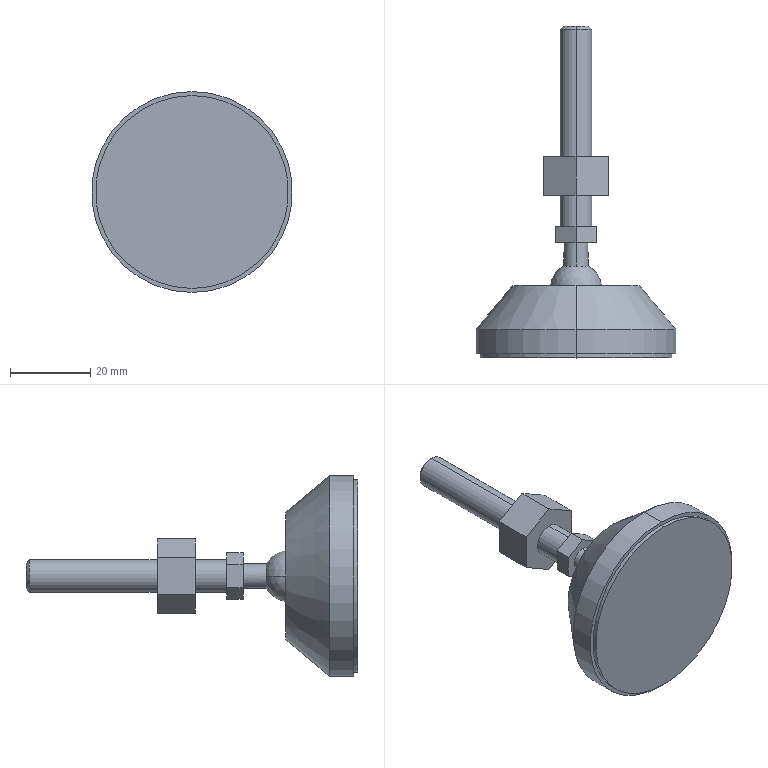Part | SolidWorks | features BaseBody 1 | 1 solid | 36 faces | box 50 x 82.6 x 50 mm | volume 33276 mm3 | plane 20 | cylinder 10 | cone 4 | sphere 2 | commonest cylinder face diameters 8 x4 6 x2 48 x2 50 x2
STEP:
#1=CARTESIAN_POINT('',(0.,7.,-25.));
#2=VERTEX_POINT('',#1);
#3=CARTESIAN_POINT('',(0.,7.,25.));
#4=VERTEX_POINT('',#3);
#5=CARTESIAN_POINT('',(0.,7.,0.));
#6=DIRECTION('',(0.,1.,0.));
#7=DIRECTION('',(0.,0.,1.));
#8=AXIS2_PLACEMENT_3D('',#5,#6,#7);
#9=CIRCLE('',#8,25.);
#10=EDGE_CURVE('',#2,#4,#9,.T.);
#11=ORIENTED_EDGE('',*,*,#10,.F.);
#12=CARTESIAN_POINT('',(0.,1.,-25.));
#13=VERTEX_POINT('',#12);
#14=CARTESIAN_POINT('',(0.,82.6,-25.));
#15=DIRECTION('',(0.,-1.,0.));
#16=VECTOR('',#15,1000.);
#17=LINE('',#14,#16);
#18=EDGE_CURVE('',#2,#13,#17,.T.);
#19=ORIENTED_EDGE('',*,*,#18,.T.);
#20=CARTESIAN_POINT('',(0.,1.,25.));
#21=VERTEX_POINT('',#20);
#22=CARTESIAN_POINT('',(0.,1.,0.));
#23=DIRECTION('',(0.,1.,0.));
#24=DIRECTION('',(0.,0.,1.));
#25=AXIS2_PLACEMENT_3D('',#22,#23,#24);
#26=CIRCLE('',#25,25.);
#27=EDGE_CURVE('',#13,#21,#26,.T.);
#28=ORIENTED_EDGE('',*,*,#27,.T.);
#29=CARTESIAN_POINT('',(0.,82.6,25.));
#30=DIRECTION('',(0.,-1.,0.));
#31=VECTOR('',#30,1000.);
#32=LINE('',#29,#31);
#33=EDGE_CURVE('',#4,#21,#32,.T.);
#34=ORIENTED_EDGE('',*,*,#33,.F.);
#35=EDGE_LOOP('',(#11,#19,#28,#34));
#36=FACE_OUTER_BOUND('',#35,.T.);
#37=CARTESIAN_POINT('',(0.,82.6,0.));
#38=DIRECTION('',(0.,-1.,0.));
#39=DIRECTION('',(0.,0.,1.));
#40=AXIS2_PLACEMENT_3D('',#37,#38,#39);
#41=CYLINDRICAL_SURFACE('',#40,25.);
#42=ADVANCED_FACE('',(#36),#41,.T.);
#43=CARTESIAN_POINT('',(0.,18.,15.77));
#44=VERTEX_POINT('',#43);
#45=CARTESIAN_POINT('',(0.,18.,-15.77));
#46=VERTEX_POINT('',#45);
#47=CARTESIAN_POINT('',(0.,18.,0.));
#48=DIRECTION('',(0.,1.,0.));
#49=DIRECTION('',(0.,0.,1.));
#50=AXIS2_PLACEMENT_3D('',#47,#48,#49);
#51=CIRCLE('',#50,15.77);
#52=EDGE_CURVE('',#44,#46,#51,.T.);
#53=ORIENTED_EDGE('',*,*,#52,.F.);
#54=CARTESIAN_POINT('',(0.,7.,25.));
#55=DIRECTION('',(0.,-0.766,0.6428));
#56=VECTOR('',#55,1000.);
#57=LINE('',#54,#56);
#58=EDGE_CURVE('',#44,#4,#57,.T.);
#59=ORIENTED_EDGE('',*,*,#58,.T.);
#60=CARTESIAN_POINT('',(0.,7.,0.));
#61=DIRECTION('',(0.,1.,0.));
#62=DIRECTION('',(0.,0.,1.));
#63=AXIS2_PLACEMENT_3D('',#60,#61,#62);
#64=CIRCLE('',#63,25.);
#65=EDGE_CURVE('',#4,#2,#64,.T.);
#66=ORIENTED_EDGE('',*,*,#65,.T.);
#67=CARTESIAN_POINT('',(0.,7.,-25.));
#68=DIRECTION('',(0.,-0.766,-0.6428));
#69=VECTOR('',#68,1000.);
#70=LINE('',#67,#69);
#71=EDGE_CURVE('',#46,#2,#70,.T.);
#72=ORIENTED_EDGE('',*,*,#71,.F.);
#73=EDGE_LOOP('',(#53,#59,#66,#72));
#74=FACE_OUTER_BOUND('',#73,.T.);
#75=CARTESIAN_POINT('',(0.,7.,0.));
#76=DIRECTION('',(0.,-1.,0.));
#77=DIRECTION('',(0.,0.,-1.));
#78=AXIS2_PLACEMENT_3D('',#75,#76,#77);
#79=CONICAL_SURFACE('',#78,25.,0.6981);
#80=ADVANCED_FACE('',(#74),#79,.T.);
#81=CARTESIAN_POINT('',(-6.35,18.,0.));
#82=VERTEX_POINT('',#81);
#83=CARTESIAN_POINT('',(6.35,18.,0.));
#84=VERTEX_POINT('',#83);
#85=CARTESIAN_POINT('',(0.,18.,0.));
#86=DIRECTION('',(0.,1.,0.));
#87=DIRECTION('',(0.,0.,1.));
#88=AXIS2_PLACEMENT_3D('',#85,#86,#87);
#89=CIRCLE('',#88,6.35);
#90=EDGE_CURVE('',#82,#84,#89,.T.);
#91=ORIENTED_EDGE('',*,*,#90,.T.);
#92=CARTESIAN_POINT('',(3.,22.853,0.));
#93=VERTEX_POINT('',#92);
#94=CARTESIAN_POINT('',(0.,17.2,0.));
#95=DIRECTION('',(0.,0.,1.));
#96=DIRECTION('',(1.,0.,0.));
#97=AXIS2_PLACEMENT_3D('',#94,#95,#96);
#98=CIRCLE('',#97,6.4);
#99=EDGE_CURVE('',#84,#93,#98,.T.);
#100=ORIENTED_EDGE('',*,*,#99,.T.);
#101=CARTESIAN_POINT('',(0.,22.853,3.));
#102=VERTEX_POINT('',#101);
#103=CARTESIAN_POINT('',(0.,22.853,0.));
#104=DIRECTION('',(0.,1.,0.));
#105=DIRECTION('',(0.,0.,1.));
#106=AXIS2_PLACEMENT_3D('',#103,#104,#105);
#107=CIRCLE('',#106,3.);
#108=EDGE_CURVE('',#102,#93,#107,.T.);
#109=ORIENTED_EDGE('',*,*,#108,.F.);
#110=CARTESIAN_POINT('',(-3.,22.853,0.));
#111=VERTEX_POINT('',#110);
#112=CARTESIAN_POINT('',(0.,22.853,0.));
#113=DIRECTION('',(0.,1.,0.));
#114=DIRECTION('',(0.,0.,1.));
#115=AXIS2_PLACEMENT_3D('',#112,#113,#114);
#116=CIRCLE('',#115,3.);
#117=EDGE_CURVE('',#111,#102,#116,.T.);
#118=ORIENTED_EDGE('',*,*,#117,.F.);
#119=CARTESIAN_POINT('',(0.,17.2,0.));
#120=DIRECTION('',(0.,0.,-1.));
#121=DIRECTION('',(-1.,0.,0.));
#122=AXIS2_PLACEMENT_3D('',#119,#120,#121);
#123=CIRCLE('',#122,6.4);
#124=EDGE_CURVE('',#82,#111,#123,.T.);
#125=ORIENTED_EDGE('',*,*,#124,.F.);
#126=EDGE_LOOP('',(#91,#100,#109,#118,#125));
#127=FACE_OUTER_BOUND('',#126,.T.);
#128=CARTESIAN_POINT('',(0.,17.2,0.));
#129=DIRECTION('',(0.,0.,1.));
#130=DIRECTION('',(-1.,0.,0.));
#131=AXIS2_PLACEMENT_3D('',#128,#129,#130);
#132=SPHERICAL_SURFACE('',#131,6.4);
#133=ADVANCED_FACE('',(#127),#132,.T.);
#134=CARTESIAN_POINT('',(0.,28.6,-3.));
#135=VERTEX_POINT('',#134);
#136=CARTESIAN_POINT('',(0.,28.6,3.));
#137=VERTEX_POINT('',#136);
#138=CARTESIAN_POINT('',(0.,28.6,0.));
#139=DIRECTION('',(0.,1.,0.));
#140=DIRECTION('',(0.,0.,1.));
#141=AXIS2_PLACEMENT_3D('',#138,#139,#140);
#142=CIRCLE('',#141,3.);
#143=EDGE_CURVE('',#135,#137,#142,.T.);
#144=ORIENTED_EDGE('',*,*,#143,.F.);
#145=CARTESIAN_POINT('',(0.,22.853,-3.));
#146=VERTEX_POINT('',#145);
#147=CARTESIAN_POINT('',(0.,82.6,-3.));
#148=DIRECTION('',(0.,-1.,0.));
#149=VECTOR('',#148,1000.);
#150=LINE('',#147,#149);
#151=EDGE_CURVE('',#135,#146,#150,.T.);
#152=ORIENTED_EDGE('',*,*,#151,.T.);
#153=CARTESIAN_POINT('',(0.,22.853,0.));
#154=DIRECTION('',(0.,1.,0.));
#155=DIRECTION('',(0.,0.,1.));
#156=AXIS2_PLACEMENT_3D('',#153,#154,#155);
#157=CIRCLE('',#156,3.);
#158=EDGE_CURVE('',#146,#111,#157,.T.);
#159=ORIENTED_EDGE('',*,*,#158,.T.);
#160=ORIENTED_EDGE('',*,*,#117,.T.);
#161=CARTESIAN_POINT('',(0.,82.6,3.));
#162=DIRECTION('',(0.,-1.,0.));
#163=VECTOR('',#162,1000.);
#164=LINE('',#161,#163);
#165=EDGE_CURVE('',#137,#102,#164,.T.);
#166=ORIENTED_EDGE('',*,*,#165,.F.);
#167=EDGE_LOOP('',(#144,#152,#159,#160,#166));
#168=FACE_OUTER_BOUND('',#167,.T.);
#169=CARTESIAN_POINT('',(0.,82.6,0.));
#170=DIRECTION('',(0.,-1.,0.));
#171=DIRECTION('',(0.,0.,1.));
#172=AXIS2_PLACEMENT_3D('',#169,#170,#171);
#173=CYLINDRICAL_SURFACE('',#172,3.);
#174=ADVANCED_FACE('',(#168),#173,.T.);
#175=CARTESIAN_POINT('',(0.,82.6,3.233));
#176=VERTEX_POINT('',#175);
#177=CARTESIAN_POINT('',(0.,82.6,-3.233));
#178=VERTEX_POINT('',#177);
#179=CARTESIAN_POINT('',(0.,82.6,0.));
#180=DIRECTION('',(0.,1.,0.));
#181=DIRECTION('',(0.,0.,1.));
#182=AXIS2_PLACEMENT_3D('',#179,#180,#181);
#183=CIRCLE('',#182,3.233);
#184=EDGE_CURVE('',#176,#178,#183,.T.);
#185=ORIENTED_EDGE('',*,*,#184,.F.);
#186=CARTESIAN_POINT('',(0.,81.833,4.));
#187=VERTEX_POINT('',#186);
#188=CARTESIAN_POINT('',(0.,81.833,4.));
#189=DIRECTION('',(0.,-0.7071,0.7071));
#190=VECTOR('',#189,1000.);
#191=LINE('',#188,#190);
#192=EDGE_CURVE('',#176,#187,#191,.T.);
#193=ORIENTED_EDGE('',*,*,#192,.T.);
#194=CARTESIAN_POINT('',(0.,81.833,-4.));
#195=VERTEX_POINT('',#194);
#196=CARTESIAN_POINT('',(0.,81.833,0.));
#197=DIRECTION('',(0.,1.,0.));
#198=DIRECTION('',(0.,0.,1.));
#199=AXIS2_PLACEMENT_3D('',#196,#197,#198);
#200=CIRCLE('',#199,4.);
#201=EDGE_CURVE('',#187,#195,#200,.T.);
#202=ORIENTED_EDGE('',*,*,#201,.T.);
#203=CARTESIAN_POINT('',(0.,81.833,-4.));
#204=DIRECTION('',(0.,-0.7071,-0.7071));
#205=VECTOR('',#204,1000.);
#206=LINE('',#203,#205);
#207=EDGE_CURVE('',#178,#195,#206,.T.);
#208=ORIENTED_EDGE('',*,*,#207,.F.);
#209=EDGE_LOOP('',(#185,#193,#202,#208));
#210=FACE_OUTER_BOUND('',#209,.T.);
#211=CARTESIAN_POINT('',(0.,81.833,0.));
#212=DIRECTION('',(0.,-1.,0.));
#213=DIRECTION('',(0.,0.,-1.));
#214=AXIS2_PLACEMENT_3D('',#211,#212,#213);
#215=CONICAL_SURFACE('',#214,4.,0.7854);
#216=ADVANCED_FACE('',(#210),#215,.T.);
#217=CARTESIAN_POINT('',(0.,81.833,0.));
#218=DIRECTION('',(0.,1.,0.));
#219=DIRECTION('',(0.,0.,1.));
#220=AXIS2_PLACEMENT_3D('',#217,#218,#219);
#221=CIRCLE('',#220,4.);
#222=EDGE_CURVE('',#195,#187,#221,.T.);
#223=ORIENTED_EDGE('',*,*,#222,.F.);
#224=CARTESIAN_POINT('',(0.,50.,-4.));
#225=VERTEX_POINT('',#224);
#226=CARTESIAN_POINT('',(0.,82.6,-4.));
#227=DIRECTION('',(0.,-1.,0.));
#228=VECTOR('',#227,1000.);
#229=LINE('',#226,#228);
#230=EDGE_CURVE('',#195,#225,#229,.T.);
#231=ORIENTED_EDGE('',*,*,#230,.T.);
#232=CARTESIAN_POINT('',(0.,50.,4.));
#233=VERTEX_POINT('',#232);
#234=CARTESIAN_POINT('',(0.,50.,0.));
#235=DIRECTION('',(0.,1.,0.));
#236=DIRECTION('',(1.,0.,0.));
#237=AXIS2_PLACEMENT_3D('',#234,#235,#236);
#238=CIRCLE('',#237,4.);
#239=EDGE_CURVE('',#225,#233,#238,.T.);
#240=ORIENTED_EDGE('',*,*,#239,.T.);
#241=CARTESIAN_POINT('',(0.,82.6,4.));
#242=DIRECTION('',(0.,-1.,0.));
#243=VECTOR('',#242,1000.);
#244=LINE('',#241,#243);
#245=EDGE_CURVE('',#187,#233,#244,.T.);
#246=ORIENTED_EDGE('',*,*,#245,.F.);
#247=EDGE_LOOP('',(#223,#231,#240,#246));
#248=FACE_OUTER_BOUND('',#247,.T.);
#249=CARTESIAN_POINT('',(0.,82.6,0.));
#250=DIRECTION('',(0.,-1.,0.));
#251=DIRECTION('',(0.,0.,1.));
#252=AXIS2_PLACEMENT_3D('',#249,#250,#251);
#253=CYLINDRICAL_SURFACE('',#252,4.);
#254=ADVANCED_FACE('',(#248),#253,.T.);
#255=CARTESIAN_POINT('',(0.,40.5,-4.));
#256=VERTEX_POINT('',#255);
#257=CARTESIAN_POINT('',(0.,40.5,4.));
#258=VERTEX_POINT('',#257);
#259=CARTESIAN_POINT('',(0.,40.5,0.));
#260=DIRECTION('',(0.,1.,0.));
#261=DIRECTION('',(1.,0.,0.));
#262=AXIS2_PLACEMENT_3D('',#259,#260,#261);
#263=CIRCLE('',#262,4.);
#264=EDGE_CURVE('',#256,#258,#263,.T.);
#265=ORIENTED_EDGE('',*,*,#264,.F.);
#266=CARTESIAN_POINT('',(0.,32.6,-4.));
#267=VERTEX_POINT('',#266);
#268=CARTESIAN_POINT('',(0.,82.6,-4.));
#269=DIRECTION('',(0.,-1.,0.));
#270=VECTOR('',#269,1000.);
#271=LINE('',#268,#270);
#272=EDGE_CURVE('',#256,#267,#271,.T.);
#273=ORIENTED_EDGE('',*,*,#272,.T.);
#274=CARTESIAN_POINT('',(0.,32.6,4.));
#275=VERTEX_POINT('',#274);
#276=CARTESIAN_POINT('',(0.,32.6,0.));
#277=DIRECTION('',(0.,1.,0.));
#278=DIRECTION('',(0.,0.,1.));
#279=AXIS2_PLACEMENT_3D('',#276,#277,#278);
#280=CIRCLE('',#279,4.);
#281=EDGE_CURVE('',#267,#275,#280,.T.);
#282=ORIENTED_EDGE('',*,*,#281,.T.);
#283=CARTESIAN_POINT('',(0.,82.6,4.));
#284=DIRECTION('',(0.,-1.,0.));
#285=VECTOR('',#284,1000.);
#286=LINE('',#283,#285);
#287=EDGE_CURVE('',#258,#275,#286,.T.);
#288=ORIENTED_EDGE('',*,*,#287,.F.);
#289=EDGE_LOOP('',(#265,#273,#282,#288));
#290=FACE_OUTER_BOUND('',#289,.T.);
#291=CARTESIAN_POINT('',(0.,82.6,0.));
#292=DIRECTION('',(0.,-1.,0.));
#293=DIRECTION('',(0.,0.,1.));
#294=AXIS2_PLACEMENT_3D('',#291,#292,#293);
#295=CYLINDRICAL_SURFACE('',#294,4.);
#296=ADVANCED_FACE('',(#290),#295,.T.);
#297=CARTESIAN_POINT('',(0.,1.,-24.));
#298=VERTEX_POINT('',#297);
#299=CARTESIAN_POINT('',(0.,1.,24.));
#300=VERTEX_POINT('',#299);
#301=CARTESIAN_POINT('',(0.,1.,0.));
#302=DIRECTION('',(0.,1.,0.));
#303=DIRECTION('',(0.,0.,1.));
#304=AXIS2_PLACEMENT_3D('',#301,#302,#303);
#305=CIRCLE('',#304,24.);
#306=EDGE_CURVE('',#298,#300,#305,.T.);
#307=ORIENTED_EDGE('',*,*,#306,.F.);
#308=CARTESIAN_POINT('',(0.,0.,-24.));
#309=VERTEX_POINT('',#308);
#310=CARTESIAN_POINT('',(0.,82.6,-24.));
#311=DIRECTION('',(0.,-1.,0.));
#312=VECTOR('',#311,1000.);
#313=LINE('',#310,#312);
#314=EDGE_CURVE('',#298,#309,#313,.T.);
#315=ORIENTED_EDGE('',*,*,#314,.T.);
#316=CARTESIAN_POINT('',(0.,0.,24.));
#317=VERTEX_POINT('',#316);
#318=CARTESIAN_POINT('',(0.,0.,0.));
#319=DIRECTION('',(0.,1.,0.));
#320=DIRECTION('',(0.,0.,1.));
#321=AXIS2_PLACEMENT_3D('',#318,#319,#320);
#322=CIRCLE('',#321,24.);
#323=EDGE_CURVE('',#309,#317,#322,.T.);
#324=ORIENTED_EDGE('',*,*,#323,.T.);
#325=CARTESIAN_POINT('',(0.,82.6,24.));
#326=DIRECTION('',(0.,-1.,0.));
#327=VECTOR('',#326,1000.);
#328=LINE('',#325,#327);
#329=EDGE_CURVE('',#300,#317,#328,.T.);
#330=ORIENTED_EDGE('',*,*,#329,.F.);
#331=EDGE_LOOP('',(#307,#315,#324,#330));
#332=FACE_OUTER_BOUND('',#331,.T.);
#333=CARTESIAN_POINT('',(0.,82.6,0.));
#334=DIRECTION('',(0.,-1.,0.));
#335=DIRECTION('',(0.,0.,1.));
#336=AXIS2_PLACEMENT_3D('',#333,#334,#335);
#337=CYLINDRICAL_SURFACE('',#336,24.);
#338=ADVANCED_FACE('',(#332),#337,.T.);
#339=CARTESIAN_POINT('',(0.,0.,0.));
#340=DIRECTION('',(0.,1.,0.));
#341=DIRECTION('',(0.,0.,1.));
#342=AXIS2_PLACEMENT_3D('',#339,#340,#341);
#343=CIRCLE('',#342,24.);
#344=EDGE_CURVE('',#317,#309,#343,.T.);
#345=ORIENTED_EDGE('',*,*,#344,.F.);
#346=ORIENTED_EDGE('',*,*,#323,.F.);
#347=EDGE_LOOP('',(#345,#346));
#348=FACE_OUTER_BOUND('',#347,.T.);
#349=CARTESIAN_POINT('',(0.,0.,0.));
#350=DIRECTION('',(0.,1.,0.));
#351=DIRECTION('',(1.,0.,0.));
#352=AXIS2_PLACEMENT_3D('',#349,#350,#351);
#353=PLANE('',#352);
#354=ADVANCED_FACE('',(#348),#353,.F.);
#355=ORIENTED_EDGE('',*,*,#314,.F.);
#356=CARTESIAN_POINT('',(0.,1.,0.));
#357=DIRECTION('',(0.,1.,0.));
#358=DIRECTION('',(0.,0.,1.));
#359=AXIS2_PLACEMENT_3D('',#356,#357,#358);
#360=CIRCLE('',#359,24.);
#361=EDGE_CURVE('',#300,#298,#360,.T.);
#362=ORIENTED_EDGE('',*,*,#361,.F.);
#363=ORIENTED_EDGE('',*,*,#329,.T.);
#364=ORIENTED_EDGE('',*,*,#344,.T.);
#365=EDGE_LOOP('',(#355,#362,#363,#364));
#366=FACE_OUTER_BOUND('',#365,.T.);
#367=CARTESIAN_POINT('',(0.,82.6,0.));
#368=DIRECTION('',(0.,-1.,0.));
#369=DIRECTION('',(0.,0.,1.));
#370=AXIS2_PLACEMENT_3D('',#367,#368,#369);
#371=CYLINDRICAL_SURFACE('',#370,24.);
#372=ADVANCED_FACE('',(#366),#371,.T.);
#373=CARTESIAN_POINT('',(-5.,28.6,2.887));
#374=VERTEX_POINT('',#373);
#375=CARTESIAN_POINT('',(0.,28.6,5.774));
#376=VERTEX_POINT('',#375);
#377=CARTESIAN_POINT('',(-5.,28.6,2.887));
#378=DIRECTION('',(0.866,0.,0.5));
#379=VECTOR('',#378,1000.);
#380=LINE('',#377,#379);
#381=EDGE_CURVE('',#374,#376,#380,.T.);
#382=ORIENTED_EDGE('',*,*,#381,.F.);
#383=CARTESIAN_POINT('',(-5.,28.6,-2.887));
#384=VERTEX_POINT('',#383);
#385=CARTESIAN_POINT('',(-5.,28.6,-2.887));
#386=DIRECTION('',(0.,0.,1.));
#387=VECTOR('',#386,1000.);
#388=LINE('',#385,#387);
#389=EDGE_CURVE('',#384,#374,#388,.T.);
#390=ORIENTED_EDGE('',*,*,#389,.F.);
#391=CARTESIAN_POINT('',(0.,28.6,-5.774));
#392=VERTEX_POINT('',#391);
#393=CARTESIAN_POINT('',(0.,28.6,-5.774));
#394=DIRECTION('',(-0.866,0.,0.5));
#395=VECTOR('',#394,1000.);
#396=LINE('',#393,#395);
#397=EDGE_CURVE('',#392,#384,#396,.T.);
#398=ORIENTED_EDGE('',*,*,#397,.F.);
#399=CARTESIAN_POINT('',(5.,28.6,-2.887));
#400=VERTEX_POINT('',#399);
#401=CARTESIAN_POINT('',(5.,28.6,-2.887));
#402=DIRECTION('',(-0.866,0.,-0.5));
#403=VECTOR('',#402,1000.);
#404=LINE('',#401,#403);
#405=EDGE_CURVE('',#400,#392,#404,.T.);
#406=ORIENTED_EDGE('',*,*,#405,.F.);
#407=CARTESIAN_POINT('',(5.,28.6,2.887));
#408=VERTEX_POINT('',#407);
#409=CARTESIAN_POINT('',(5.,28.6,2.887));
#410=DIRECTION('',(0.,0.,-1.));
#411=VECTOR('',#410,1000.);
#412=LINE('',#409,#411);
#413=EDGE_CURVE('',#408,#400,#412,.T.);
#414=ORIENTED_EDGE('',*,*,#413,.F.);
#415=CARTESIAN_POINT('',(0.,28.6,5.774));
#416=DIRECTION('',(0.866,0.,-0.5));
#417=VECTOR('',#416,1000.);
#418=LINE('',#415,#417);
#419=EDGE_CURVE('',#376,#408,#418,.T.);
#420=ORIENTED_EDGE('',*,*,#419,.F.);
#421=EDGE_LOOP('',(#382,#390,#398,#406,#414,#420));
#422=FACE_OUTER_BOUND('',#421,.T.);
#423=CARTESIAN_POINT('',(0.,28.6,0.));
#424=DIRECTION('',(0.,1.,0.));
#425=DIRECTION('',(0.,0.,1.));
#426=AXIS2_PLACEMENT_3D('',#423,#424,#425);
#427=CIRCLE('',#426,3.);
#428=EDGE_CURVE('',#137,#135,#427,.T.);
#429=ORIENTED_EDGE('',*,*,#428,.T.);
#430=ORIENTED_EDGE('',*,*,#143,.T.);
#431=EDGE_LOOP('',(#429,#430));
#432=FACE_BOUND('',#431,.T.);
#433=CARTESIAN_POINT('',(-3.,28.6,0.));
#434=DIRECTION('',(0.,1.,0.));
#435=DIRECTION('',(1.,0.,0.));
#436=AXIS2_PLACEMENT_3D('',#433,#434,#435);
#437=PLANE('',#436);
#438=ADVANCED_FACE('',(#422,#432),#437,.F.);
#439=ORIENTED_EDGE('',*,*,#272,.F.);
#440=CARTESIAN_POINT('',(0.,40.5,0.));
#441=DIRECTION('',(0.,1.,0.));
#442=DIRECTION('',(1.,0.,0.));
#443=AXIS2_PLACEMENT_3D('',#440,#441,#442);
#444=CIRCLE('',#443,4.);
#445=EDGE_CURVE('',#258,#256,#444,.T.);
#446=ORIENTED_EDGE('',*,*,#445,.F.);
#447=ORIENTED_EDGE('',*,*,#287,.T.);
#448=CARTESIAN_POINT('',(0.,32.6,0.));
#449=DIRECTION('',(0.,1.,0.));
#450=DIRECTION('',(0.,0.,1.));
#451=AXIS2_PLACEMENT_3D('',#448,#449,#450);
#452=CIRCLE('',#451,4.);
#453=EDGE_CURVE('',#275,#267,#452,.T.);
#454=ORIENTED_EDGE('',*,*,#453,.T.);
#455=EDGE_LOOP('',(#439,#446,#447,#454));
#456=FACE_OUTER_BOUND('',#455,.T.);
#457=CARTESIAN_POINT('',(0.,82.6,0.));
#458=DIRECTION('',(0.,-1.,0.));
#459=DIRECTION('',(0.,0.,1.));
#460=AXIS2_PLACEMENT_3D('',#457,#458,#459);
#461=CYLINDRICAL_SURFACE('',#460,4.);
#462=ADVANCED_FACE('',(#456),#461,.T.);
#463=ORIENTED_EDGE('',*,*,#230,.F.);
#464=ORIENTED_EDGE('',*,*,#201,.F.);
#465=ORIENTED_EDGE('',*,*,#245,.T.);
#466=CARTESIAN_POINT('',(0.,50.,0.));
#467=DIRECTION('',(0.,1.,0.));
#468=DIRECTION('',(1.,0.,0.));
#469=AXIS2_PLACEMENT_3D('',#466,#467,#468);
#470=CIRCLE('',#469,4.);
#471=EDGE_CURVE('',#233,#225,#470,.T.);
#472=ORIENTED_EDGE('',*,*,#471,.T.);
#473=EDGE_LOOP('',(#463,#464,#465,#472));
#474=FACE_OUTER_BOUND('',#473,.T.);
#475=CARTESIAN_POINT('',(0.,82.6,0.));
#476=DIRECTION('',(0.,-1.,0.));
#477=DIRECTION('',(0.,0.,1.));
#478=AXIS2_PLACEMENT_3D('',#475,#476,#477);
#479=CYLINDRICAL_SURFACE('',#478,4.);
#480=ADVANCED_FACE('',(#474),#479,.T.);
#481=ORIENTED_EDGE('',*,*,#192,.F.);
#482=CARTESIAN_POINT('',(0.,82.6,0.));
#483=DIRECTION('',(0.,1.,0.));
#484=DIRECTION('',(0.,0.,1.));
#485=AXIS2_PLACEMENT_3D('',#482,#483,#484);
#486=CIRCLE('',#485,3.233);
#487=EDGE_CURVE('',#178,#176,#486,.T.);
#488=ORIENTED_EDGE('',*,*,#487,.F.);
#489=ORIENTED_EDGE('',*,*,#207,.T.);
#490=ORIENTED_EDGE('',*,*,#222,.T.);
#491=EDGE_LOOP('',(#481,#488,#489,#490));
#492=FACE_OUTER_BOUND('',#491,.T.);
#493=CARTESIAN_POINT('',(0.,81.833,0.));
#494=DIRECTION('',(0.,-1.,0.));
#495=DIRECTION('',(0.,0.,-1.));
#496=AXIS2_PLACEMENT_3D('',#493,#494,#495);
#497=CONICAL_SURFACE('',#496,4.,0.7854);
#498=ADVANCED_FACE('',(#492),#497,.T.);
#499=CARTESIAN_POINT('',(-8.,50.,-4.619));
#500=VERTEX_POINT('',#499);
#501=CARTESIAN_POINT('',(-8.,50.,4.619));
#502=VERTEX_POINT('',#501);
#503=CARTESIAN_POINT('',(-8.,50.,-4.619));
#504=DIRECTION('',(0.,0.,1.));
#505=VECTOR('',#504,1000.);
#506=LINE('',#503,#505);
#507=EDGE_CURVE('',#500,#502,#506,.T.);
#508=ORIENTED_EDGE('',*,*,#507,.T.);
#509=CARTESIAN_POINT('',(0.,50.,9.238));
#510=VERTEX_POINT('',#509);
#511=CARTESIAN_POINT('',(-8.,50.,4.619));
#512=DIRECTION('',(0.866,0.,0.5));
#513=VECTOR('',#512,1000.);
#514=LINE('',#511,#513);
#515=EDGE_CURVE('',#502,#510,#514,.T.);
#516=ORIENTED_EDGE('',*,*,#515,.T.);
#517=CARTESIAN_POINT('',(8.,50.,4.619));
#518=VERTEX_POINT('',#517);
#519=CARTESIAN_POINT('',(0.,50.,9.238));
#520=DIRECTION('',(0.866,0.,-0.5));
#521=VECTOR('',#520,1000.);
#522=LINE('',#519,#521);
#523=EDGE_CURVE('',#510,#518,#522,.T.);
#524=ORIENTED_EDGE('',*,*,#523,.T.);
#525=CARTESIAN_POINT('',(8.,50.,-4.619));
#526=VERTEX_POINT('',#525);
#527=CARTESIAN_POINT('',(8.,50.,4.619));
#528=DIRECTION('',(0.,0.,-1.));
#529=VECTOR('',#528,1000.);
#530=LINE('',#527,#529);
#531=EDGE_CURVE('',#518,#526,#530,.T.);
#532=ORIENTED_EDGE('',*,*,#531,.T.);
#533=CARTESIAN_POINT('',(0.,50.,-9.238));
#534=VERTEX_POINT('',#533);
#535=CARTESIAN_POINT('',(8.,50.,-4.619));
#536=DIRECTION('',(-0.866,0.,-0.5));
#537=VECTOR('',#536,1000.);
#538=LINE('',#535,#537);
#539=EDGE_CURVE('',#526,#534,#538,.T.);
#540=ORIENTED_EDGE('',*,*,#539,.T.);
#541=CARTESIAN_POINT('',(0.,50.,-9.238));
#542=DIRECTION('',(-0.866,0.,0.5));
#543=VECTOR('',#542,1000.);
#544=LINE('',#541,#543);
#545=EDGE_CURVE('',#534,#500,#544,.T.);
#546=ORIENTED_EDGE('',*,*,#545,.T.);
#547=EDGE_LOOP('',(#508,#516,#524,#532,#540,#546));
#548=FACE_OUTER_BOUND('',#547,.T.);
#549=ORIENTED_EDGE('',*,*,#471,.F.);
#550=ORIENTED_EDGE('',*,*,#239,.F.);
#551=EDGE_LOOP('',(#549,#550));
#552=FACE_BOUND('',#551,.T.);
#553=CARTESIAN_POINT('',(0.,50.,0.));
#554=DIRECTION('',(0.,1.,0.));
#555=DIRECTION('',(1.,0.,0.));
#556=AXIS2_PLACEMENT_3D('',#553,#554,#555);
#557=PLANE('',#556);
#558=ADVANCED_FACE('',(#548,#552),#557,.T.);
#559=ORIENTED_EDGE('',*,*,#523,.F.);
#560=CARTESIAN_POINT('',(0.,40.5,9.238));
#561=VERTEX_POINT('',#560);
#562=CARTESIAN_POINT('',(0.,40.5,9.238));
#563=DIRECTION('',(0.,1.,0.));
#564=VECTOR('',#563,1000.);
#565=LINE('',#562,#564);
#566=EDGE_CURVE('',#561,#510,#565,.T.);
#567=ORIENTED_EDGE('',*,*,#566,.F.);
#568=CARTESIAN_POINT('',(8.,40.5,4.619));
#569=VERTEX_POINT('',#568);
#570=CARTESIAN_POINT('',(0.,40.5,9.238));
#571=DIRECTION('',(0.866,0.,-0.5));
#572=VECTOR('',#571,1000.);
#573=LINE('',#570,#572);
#574=EDGE_CURVE('',#561,#569,#573,.T.);
#575=ORIENTED_EDGE('',*,*,#574,.T.);
#576=CARTESIAN_POINT('',(8.,40.5,4.619));
#577=DIRECTION('',(0.,1.,0.));
#578=VECTOR('',#577,1000.);
#579=LINE('',#576,#578);
#580=EDGE_CURVE('',#569,#518,#579,.T.);
#581=ORIENTED_EDGE('',*,*,#580,.T.);
#582=EDGE_LOOP('',(#559,#567,#575,#581));
#583=FACE_OUTER_BOUND('',#582,.T.);
#584=CARTESIAN_POINT('',(0.,40.5,9.238));
#585=DIRECTION('',(0.5,0.,0.866));
#586=DIRECTION('',(0.,-1.,0.));
#587=AXIS2_PLACEMENT_3D('',#584,#585,#586);
#588=PLANE('',#587);
#589=ADVANCED_FACE('',(#583),#588,.T.);
#590=ORIENTED_EDGE('',*,*,#531,.F.);
#591=ORIENTED_EDGE('',*,*,#580,.F.);
#592=CARTESIAN_POINT('',(8.,40.5,-4.619));
#593=VERTEX_POINT('',#592);
#594=CARTESIAN_POINT('',(8.,40.5,4.619));
#595=DIRECTION('',(0.,0.,-1.));
#596=VECTOR('',#595,1000.);
#597=LINE('',#594,#596);
#598=EDGE_CURVE('',#569,#593,#597,.T.);
#599=ORIENTED_EDGE('',*,*,#598,.T.);
#600=CARTESIAN_POINT('',(8.,40.5,-4.619));
#601=DIRECTION('',(0.,1.,0.));
#602=VECTOR('',#601,1000.);
#603=LINE('',#600,#602);
#604=EDGE_CURVE('',#593,#526,#603,.T.);
#605=ORIENTED_EDGE('',*,*,#604,.T.);
#606=EDGE_LOOP('',(#590,#591,#599,#605));
#607=FACE_OUTER_BOUND('',#606,.T.);
#608=CARTESIAN_POINT('',(8.,40.5,4.619));
#609=DIRECTION('',(1.,0.,0.));
#610=DIRECTION('',(0.,1.,0.));
#611=AXIS2_PLACEMENT_3D('',#608,#609,#610);
#612=PLANE('',#611);
#613=ADVANCED_FACE('',(#607),#612,.T.);
#614=ORIENTED_EDGE('',*,*,#515,.F.);
#615=CARTESIAN_POINT('',(-8.,40.5,4.619));
#616=VERTEX_POINT('',#615);
#617=CARTESIAN_POINT('',(-8.,40.5,4.619));
#618=DIRECTION('',(0.,1.,0.));
#619=VECTOR('',#618,1000.);
#620=LINE('',#617,#619);
#621=EDGE_CURVE('',#616,#502,#620,.T.);
#622=ORIENTED_EDGE('',*,*,#621,.F.);
#623=CARTESIAN_POINT('',(-8.,40.5,4.619));
#624=DIRECTION('',(0.866,0.,0.5));
#625=VECTOR('',#624,1000.);
#626=LINE('',#623,#625);
#627=EDGE_CURVE('',#616,#561,#626,.T.);
#628=ORIENTED_EDGE('',*,*,#627,.T.);
#629=ORIENTED_EDGE('',*,*,#566,.T.);
#630=EDGE_LOOP('',(#614,#622,#628,#629));
#631=FACE_OUTER_BOUND('',#630,.T.);
#632=CARTESIAN_POINT('',(-8.,40.5,4.619));
#633=DIRECTION('',(-0.5,0.,0.866));
#634=DIRECTION('',(0.,1.,0.));
#635=AXIS2_PLACEMENT_3D('',#632,#633,#634);
#636=PLANE('',#635);
#637=ADVANCED_FACE('',(#631),#636,.T.);
#638=ORIENTED_EDGE('',*,*,#507,.F.);
#639=CARTESIAN_POINT('',(-8.,40.5,-4.619));
#640=VERTEX_POINT('',#639);
#641=CARTESIAN_POINT('',(-8.,40.5,-4.619));
#642=DIRECTION('',(0.,1.,0.));
#643=VECTOR('',#642,1000.);
#644=LINE('',#641,#643);
#645=EDGE_CURVE('',#640,#500,#644,.T.);
#646=ORIENTED_EDGE('',*,*,#645,.F.);
#647=CARTESIAN_POINT('',(-8.,40.5,-4.619));
#648=DIRECTION('',(0.,0.,1.));
#649=VECTOR('',#648,1000.);
#650=LINE('',#647,#649);
#651=EDGE_CURVE('',#640,#616,#650,.T.);
#652=ORIENTED_EDGE('',*,*,#651,.T.);
#653=ORIENTED_EDGE('',*,*,#621,.T.);
#654=EDGE_LOOP('',(#638,#646,#652,#653));
#655=FACE_OUTER_BOUND('',#654,.T.);
#656=CARTESIAN_POINT('',(-8.,40.5,-4.619));
#657=DIRECTION('',(-1.,0.,0.));
#658=DIRECTION('',(0.,0.,1.));
#659=AXIS2_PLACEMENT_3D('',#656,#657,#658);
#660=PLANE('',#659);
#661=ADVANCED_FACE('',(#655),#660,.T.);
#662=CARTESIAN_POINT('',(5.,32.6,2.887));
#663=VERTEX_POINT('',#662);
#664=CARTESIAN_POINT('',(5.,32.6,-2.887));
#665=VERTEX_POINT('',#664);
#666=CARTESIAN_POINT('',(5.,32.6,2.887));
#667=DIRECTION('',(0.,0.,-1.));
#668=VECTOR('',#667,1000.);
#669=LINE('',#666,#668);
#670=EDGE_CURVE('',#663,#665,#669,.T.);
#671=ORIENTED_EDGE('',*,*,#670,.F.);
#672=CARTESIAN_POINT('',(5.,28.6,2.887));
#673=DIRECTION('',(0.,1.,0.));
#674=VECTOR('',#673,1000.);
#675=LINE('',#672,#674);
#676=EDGE_CURVE('',#408,#663,#675,.T.);
#677=ORIENTED_EDGE('',*,*,#676,.F.);
#678=ORIENTED_EDGE('',*,*,#413,.T.);
#679=CARTESIAN_POINT('',(5.,28.6,-2.887));
#680=DIRECTION('',(0.,1.,0.));
#681=VECTOR('',#680,1000.);
#682=LINE('',#679,#681);
#683=EDGE_CURVE('',#400,#665,#682,.T.);
#684=ORIENTED_EDGE('',*,*,#683,.T.);
#685=EDGE_LOOP('',(#671,#677,#678,#684));
#686=FACE_OUTER_BOUND('',#685,.T.);
#687=CARTESIAN_POINT('',(5.,28.6,2.887));
#688=DIRECTION('',(1.,0.,0.));
#689=DIRECTION('',(0.,1.,0.));
#690=AXIS2_PLACEMENT_3D('',#687,#688,#689);
#691=PLANE('',#690);
#692=ADVANCED_FACE('',(#686),#691,.T.);
#693=CARTESIAN_POINT('',(0.,32.6,5.774));
#694=VERTEX_POINT('',#693);
#695=CARTESIAN_POINT('',(0.,32.6,5.774));
#696=DIRECTION('',(0.866,0.,-0.5));
#697=VECTOR('',#696,1000.);
#698=LINE('',#695,#697);
#699=EDGE_CURVE('',#694,#663,#698,.T.);
#700=ORIENTED_EDGE('',*,*,#699,.F.);
#701=CARTESIAN_POINT('',(0.,28.6,5.774));
#702=DIRECTION('',(0.,1.,0.));
#703=VECTOR('',#702,1000.);
#704=LINE('',#701,#703);
#705=EDGE_CURVE('',#376,#694,#704,.T.);
#706=ORIENTED_EDGE('',*,*,#705,.F.);
#707=ORIENTED_EDGE('',*,*,#419,.T.);
#708=ORIENTED_EDGE('',*,*,#676,.T.);
#709=EDGE_LOOP('',(#700,#706,#707,#708));
#710=FACE_OUTER_BOUND('',#709,.T.);
#711=CARTESIAN_POINT('',(0.,28.6,5.774));
#712=DIRECTION('',(0.5,0.,0.866));
#713=DIRECTION('',(0.,-1.,0.));
#714=AXIS2_PLACEMENT_3D('',#711,#712,#713);
#715=PLANE('',#714);
#716=ADVANCED_FACE('',(#710),#715,.T.);
#717=CARTESIAN_POINT('',(-5.,32.6,2.887));
#718=VERTEX_POINT('',#717);
#719=CARTESIAN_POINT('',(-5.,32.6,2.887));
#720=DIRECTION('',(0.866,0.,0.5));
#721=VECTOR('',#720,1000.);
#722=LINE('',#719,#721);
#723=EDGE_CURVE('',#718,#694,#722,.T.);
#724=ORIENTED_EDGE('',*,*,#723,.F.);
#725=CARTESIAN_POINT('',(-5.,28.6,2.887));
#726=DIRECTION('',(0.,1.,0.));
#727=VECTOR('',#726,1000.);
#728=LINE('',#725,#727);
#729=EDGE_CURVE('',#374,#718,#728,.T.);
#730=ORIENTED_EDGE('',*,*,#729,.F.);
#731=ORIENTED_EDGE('',*,*,#381,.T.);
#732=ORIENTED_EDGE('',*,*,#705,.T.);
#733=EDGE_LOOP('',(#724,#730,#731,#732));
#734=FACE_OUTER_BOUND('',#733,.T.);
#735=CARTESIAN_POINT('',(-5.,28.6,2.887));
#736=DIRECTION('',(-0.5,0.,0.866));
#737=DIRECTION('',(0.,1.,0.));
#738=AXIS2_PLACEMENT_3D('',#735,#736,#737);
#739=PLANE('',#738);
#740=ADVANCED_FACE('',(#734),#739,.T.);
#741=CARTESIAN_POINT('',(-5.,32.6,-2.887));
#742=VERTEX_POINT('',#741);
#743=CARTESIAN_POINT('',(-5.,32.6,0.));
#744=DIRECTION('',(0.,0.,-1.));
#745=VECTOR('',#744,1000.);
#746=LINE('',#743,#745);
#747=EDGE_CURVE('',#718,#742,#746,.T.);
#748=ORIENTED_EDGE('',*,*,#747,.T.);
#749=CARTESIAN_POINT('',(-5.,28.6,-2.887));
#750=DIRECTION('',(0.,1.,0.));
#751=VECTOR('',#750,1000.);
#752=LINE('',#749,#751);
#753=EDGE_CURVE('',#384,#742,#752,.T.);
#754=ORIENTED_EDGE('',*,*,#753,.F.);
#755=ORIENTED_EDGE('',*,*,#389,.T.);
#756=ORIENTED_EDGE('',*,*,#729,.T.);
#757=EDGE_LOOP('',(#748,#754,#755,#756));
#758=FACE_OUTER_BOUND('',#757,.T.);
#759=CARTESIAN_POINT('',(-5.,28.6,-2.887));
#760=DIRECTION('',(-1.,0.,0.));
#761=DIRECTION('',(0.,0.,1.));
#762=AXIS2_PLACEMENT_3D('',#759,#760,#761);
#763=PLANE('',#762);
#764=ADVANCED_FACE('',(#758),#763,.T.);
#765=CARTESIAN_POINT('',(0.,32.6,-5.774));
#766=VERTEX_POINT('',#765);
#767=CARTESIAN_POINT('',(0.,32.6,-5.774));
#768=DIRECTION('',(-0.866,0.,0.5));
#769=VECTOR('',#768,1000.);
#770=LINE('',#767,#769);
#771=EDGE_CURVE('',#766,#742,#770,.T.);
#772=ORIENTED_EDGE('',*,*,#771,.F.);
#773=CARTESIAN_POINT('',(0.,28.6,-5.774));
#774=DIRECTION('',(0.,1.,0.));
#775=VECTOR('',#774,1000.);
#776=LINE('',#773,#775);
#777=EDGE_CURVE('',#392,#766,#776,.T.);
#778=ORIENTED_EDGE('',*,*,#777,.F.);
#779=ORIENTED_EDGE('',*,*,#397,.T.);
#780=ORIENTED_EDGE('',*,*,#753,.T.);
#781=EDGE_LOOP('',(#772,#778,#779,#780));
#782=FACE_OUTER_BOUND('',#781,.T.);
#783=CARTESIAN_POINT('',(0.,28.6,-5.774));
#784=DIRECTION('',(-0.5,0.,-0.866));
#785=DIRECTION('',(-0.866,0.,0.5));
#786=AXIS2_PLACEMENT_3D('',#783,#784,#785);
#787=PLANE('',#786);
#788=ADVANCED_FACE('',(#782),#787,.T.);
#789=CARTESIAN_POINT('',(5.,32.6,-2.887));
#790=DIRECTION('',(-0.866,0.,-0.5));
#791=VECTOR('',#790,1000.);
#792=LINE('',#789,#791);
#793=EDGE_CURVE('',#665,#766,#792,.T.);
#794=ORIENTED_EDGE('',*,*,#793,.F.);
#795=ORIENTED_EDGE('',*,*,#683,.F.);
#796=ORIENTED_EDGE('',*,*,#405,.T.);
#797=ORIENTED_EDGE('',*,*,#777,.T.);
#798=EDGE_LOOP('',(#794,#795,#796,#797));
#799=FACE_OUTER_BOUND('',#798,.T.);
#800=CARTESIAN_POINT('',(5.,28.6,-2.887));
#801=DIRECTION('',(0.5,0.,-0.866));
#802=DIRECTION('',(0.,-1.,0.));
#803=AXIS2_PLACEMENT_3D('',#800,#801,#802);
#804=PLANE('',#803);
#805=ADVANCED_FACE('',(#799),#804,.T.);
#806=ORIENTED_EDGE('',*,*,#487,.T.);
#807=ORIENTED_EDGE('',*,*,#184,.T.);
#808=EDGE_LOOP('',(#806,#807));
#809=FACE_OUTER_BOUND('',#808,.T.);
#810=CARTESIAN_POINT('',(-3.233,82.6,0.));
#811=DIRECTION('',(0.,-1.,0.));
#812=DIRECTION('',(0.,0.,-1.));
#813=AXIS2_PLACEMENT_3D('',#810,#811,#812);
#814=PLANE('',#813);
#815=ADVANCED_FACE('',(#809),#814,.F.);
#816=ORIENTED_EDGE('',*,*,#651,.F.);
#817=CARTESIAN_POINT('',(0.,40.5,-9.238));
#818=VERTEX_POINT('',#817);
#819=CARTESIAN_POINT('',(0.,40.5,-9.238));
#820=DIRECTION('',(-0.866,0.,0.5));
#821=VECTOR('',#820,1000.);
#822=LINE('',#819,#821);
#823=EDGE_CURVE('',#818,#640,#822,.T.);
#824=ORIENTED_EDGE('',*,*,#823,.F.);
#825=CARTESIAN_POINT('',(8.,40.5,-4.619));
#826=DIRECTION('',(-0.866,0.,-0.5));
#827=VECTOR('',#826,1000.);
#828=LINE('',#825,#827);
#829=EDGE_CURVE('',#593,#818,#828,.T.);
#830=ORIENTED_EDGE('',*,*,#829,.F.);
#831=ORIENTED_EDGE('',*,*,#598,.F.);
#832=ORIENTED_EDGE('',*,*,#574,.F.);
#833=ORIENTED_EDGE('',*,*,#627,.F.);
#834=EDGE_LOOP('',(#816,#824,#830,#831,#832,#833));
#835=FACE_OUTER_BOUND('',#834,.T.);
#836=ORIENTED_EDGE('',*,*,#445,.T.);
#837=ORIENTED_EDGE('',*,*,#264,.T.);
#838=EDGE_LOOP('',(#836,#837));
#839=FACE_BOUND('',#838,.T.);
#840=CARTESIAN_POINT('',(0.,40.5,0.));
#841=DIRECTION('',(0.,1.,0.));
#842=DIRECTION('',(1.,0.,0.));
#843=AXIS2_PLACEMENT_3D('',#840,#841,#842);
#844=PLANE('',#843);
#845=ADVANCED_FACE('',(#835,#839),#844,.F.);
#846=ORIENTED_EDGE('',*,*,#545,.F.);
#847=CARTESIAN_POINT('',(0.,40.5,-9.238));
#848=DIRECTION('',(0.,1.,0.));
#849=VECTOR('',#848,1000.);
#850=LINE('',#847,#849);
#851=EDGE_CURVE('',#818,#534,#850,.T.);
#852=ORIENTED_EDGE('',*,*,#851,.F.);
#853=ORIENTED_EDGE('',*,*,#823,.T.);
#854=ORIENTED_EDGE('',*,*,#645,.T.);
#855=EDGE_LOOP('',(#846,#852,#853,#854));
#856=FACE_OUTER_BOUND('',#855,.T.);
#857=CARTESIAN_POINT('',(0.,40.5,-9.238));
#858=DIRECTION('',(-0.5,0.,-0.866));
#859=DIRECTION('',(-0.866,0.,0.5));
#860=AXIS2_PLACEMENT_3D('',#857,#858,#859);
#861=PLANE('',#860);
#862=ADVANCED_FACE('',(#856),#861,.T.);
#863=ORIENTED_EDGE('',*,*,#539,.F.);
#864=ORIENTED_EDGE('',*,*,#604,.F.);
#865=ORIENTED_EDGE('',*,*,#829,.T.);
#866=ORIENTED_EDGE('',*,*,#851,.T.);
#867=EDGE_LOOP('',(#863,#864,#865,#866));
#868=FACE_OUTER_BOUND('',#867,.T.);
#869=CARTESIAN_POINT('',(8.,40.5,-4.619));
#870=DIRECTION('',(0.5,0.,-0.866));
#871=DIRECTION('',(0.,-1.,0.));
#872=AXIS2_PLACEMENT_3D('',#869,#870,#871);
#873=PLANE('',#872);
#874=ADVANCED_FACE('',(#868),#873,.T.);
#875=ORIENTED_EDGE('',*,*,#670,.T.);
#876=ORIENTED_EDGE('',*,*,#793,.T.);
#877=ORIENTED_EDGE('',*,*,#771,.T.);
#878=ORIENTED_EDGE('',*,*,#747,.F.);
#879=ORIENTED_EDGE('',*,*,#723,.T.);
#880=ORIENTED_EDGE('',*,*,#699,.T.);
#881=EDGE_LOOP('',(#875,#876,#877,#878,#879,#880));
#882=FACE_OUTER_BOUND('',#881,.T.);
#883=ORIENTED_EDGE('',*,*,#453,.F.);
#884=ORIENTED_EDGE('',*,*,#281,.F.);
#885=EDGE_LOOP('',(#883,#884));
#886=FACE_BOUND('',#885,.T.);
#887=CARTESIAN_POINT('',(-6.4,32.6,0.));
#888=DIRECTION('',(0.,-1.,0.));
#889=DIRECTION('',(0.,0.,-1.));
#890=AXIS2_PLACEMENT_3D('',#887,#888,#889);
#891=PLANE('',#890);
#892=ADVANCED_FACE('',(#882,#886),#891,.F.);
#893=ORIENTED_EDGE('',*,*,#151,.F.);
#894=ORIENTED_EDGE('',*,*,#428,.F.);
#895=ORIENTED_EDGE('',*,*,#165,.T.);
#896=ORIENTED_EDGE('',*,*,#108,.T.);
#897=CARTESIAN_POINT('',(0.,22.853,0.));
#898=DIRECTION('',(0.,1.,0.));
#899=DIRECTION('',(0.,0.,1.));
#900=AXIS2_PLACEMENT_3D('',#897,#898,#899);
#901=CIRCLE('',#900,3.);
#902=EDGE_CURVE('',#93,#146,#901,.T.);
#903=ORIENTED_EDGE('',*,*,#902,.T.);
#904=EDGE_LOOP('',(#893,#894,#895,#896,#903));
#905=FACE_OUTER_BOUND('',#904,.T.);
#906=CARTESIAN_POINT('',(0.,82.6,0.));
#907=DIRECTION('',(0.,-1.,0.));
#908=DIRECTION('',(0.,0.,1.));
#909=AXIS2_PLACEMENT_3D('',#906,#907,#908);
#910=CYLINDRICAL_SURFACE('',#909,3.);
#911=ADVANCED_FACE('',(#905),#910,.T.);
#912=ORIENTED_EDGE('',*,*,#99,.F.);
#913=CARTESIAN_POINT('',(0.,18.,0.));
#914=DIRECTION('',(0.,1.,0.));
#915=DIRECTION('',(0.,0.,1.));
#916=AXIS2_PLACEMENT_3D('',#913,#914,#915);
#917=CIRCLE('',#916,6.35);
#918=EDGE_CURVE('',#84,#82,#917,.T.);
#919=ORIENTED_EDGE('',*,*,#918,.T.);
#920=ORIENTED_EDGE('',*,*,#124,.T.);
#921=ORIENTED_EDGE('',*,*,#158,.F.);
#922=ORIENTED_EDGE('',*,*,#902,.F.);
#923=EDGE_LOOP('',(#912,#919,#920,#921,#922));
#924=FACE_OUTER_BOUND('',#923,.T.);
#925=CARTESIAN_POINT('',(0.,17.2,0.));
#926=DIRECTION('',(0.,0.,1.));
#927=DIRECTION('',(-1.,0.,0.));
#928=AXIS2_PLACEMENT_3D('',#925,#926,#927);
#929=SPHERICAL_SURFACE('',#928,6.4);
#930=ADVANCED_FACE('',(#924),#929,.T.);
#931=CARTESIAN_POINT('',(0.,18.,0.));
#932=DIRECTION('',(0.,1.,0.));
#933=DIRECTION('',(0.,0.,1.));
#934=AXIS2_PLACEMENT_3D('',#931,#932,#933);
#935=CIRCLE('',#934,15.77);
#936=EDGE_CURVE('',#46,#44,#935,.T.);
#937=ORIENTED_EDGE('',*,*,#936,.T.);
#938=ORIENTED_EDGE('',*,*,#52,.T.);
#939=EDGE_LOOP('',(#937,#938));
#940=FACE_OUTER_BOUND('',#939,.T.);
#941=ORIENTED_EDGE('',*,*,#90,.F.);
#942=ORIENTED_EDGE('',*,*,#918,.F.);
#943=EDGE_LOOP('',(#941,#942));
#944=FACE_BOUND('',#943,.T.);
#945=CARTESIAN_POINT('',(-15.77,18.,0.));
#946=DIRECTION('',(0.,-1.,0.));
#947=DIRECTION('',(0.,0.,-1.));
#948=AXIS2_PLACEMENT_3D('',#945,#946,#947);
#949=PLANE('',#948);
#950=ADVANCED_FACE('',(#940,#944),#949,.F.);
#951=ORIENTED_EDGE('',*,*,#58,.F.);
#952=ORIENTED_EDGE('',*,*,#936,.F.);
#953=ORIENTED_EDGE('',*,*,#71,.T.);
#954=ORIENTED_EDGE('',*,*,#10,.T.);
#955=EDGE_LOOP('',(#951,#952,#953,#954));
#956=FACE_OUTER_BOUND('',#955,.T.);
#957=CARTESIAN_POINT('',(0.,7.,0.));
#958=DIRECTION('',(0.,-1.,0.));
#959=DIRECTION('',(0.,0.,-1.));
#960=AXIS2_PLACEMENT_3D('',#957,#958,#959);
#961=CONICAL_SURFACE('',#960,25.,0.6981);
#962=ADVANCED_FACE('',(#956),#961,.T.);
#963=ORIENTED_EDGE('',*,*,#18,.F.);
#964=ORIENTED_EDGE('',*,*,#65,.F.);
#965=ORIENTED_EDGE('',*,*,#33,.T.);
#966=CARTESIAN_POINT('',(0.,1.,0.));
#967=DIRECTION('',(0.,1.,0.));
#968=DIRECTION('',(0.,0.,1.));
#969=AXIS2_PLACEMENT_3D('',#966,#967,#968);
#970=CIRCLE('',#969,25.);
#971=EDGE_CURVE('',#21,#13,#970,.T.);
#972=ORIENTED_EDGE('',*,*,#971,.T.);
#973=EDGE_LOOP('',(#963,#964,#965,#972));
#974=FACE_OUTER_BOUND('',#973,.T.);
#975=CARTESIAN_POINT('',(0.,82.6,0.));
#976=DIRECTION('',(0.,-1.,0.));
#977=DIRECTION('',(0.,0.,1.));
#978=AXIS2_PLACEMENT_3D('',#975,#976,#977);
#979=CYLINDRICAL_SURFACE('',#978,25.);
#980=ADVANCED_FACE('',(#974),#979,.T.);
#981=ORIENTED_EDGE('',*,*,#971,.F.);
#982=ORIENTED_EDGE('',*,*,#27,.F.);
#983=EDGE_LOOP('',(#981,#982));
#984=FACE_OUTER_BOUND('',#983,.T.);
#985=ORIENTED_EDGE('',*,*,#361,.T.);
#986=ORIENTED_EDGE('',*,*,#306,.T.);
#987=EDGE_LOOP('',(#985,#986));
#988=FACE_BOUND('',#987,.T.);
#989=CARTESIAN_POINT('',(-24.,1.,0.));
#990=DIRECTION('',(0.,1.,0.));
#991=DIRECTION('',(1.,0.,0.));
#992=AXIS2_PLACEMENT_3D('',#989,#990,#991);
#993=PLANE('',#992);
#994=ADVANCED_FACE('',(#984,#988),#993,.F.);
#995=CLOSED_SHELL('',(#42,#80,#133,#174,#216,#254,#296,#338,#354,#372,#438,#462,#480,#498,#558,#589,#613,#637,#661,#692,#716,#740,#764,#788,#805,#815,#845,#862,#874,#892,#911,#930,#950,#962,#980,#994));
#996=MANIFOLD_SOLID_BREP('',#995);
#997=CARTESIAN_POINT('',(0.,0.,0.));
#998=DIRECTION('',(0.,0.,1.));
#999=DIRECTION('',(1.,0.,0.));
#1000=AXIS2_PLACEMENT_3D('',#997,#998,#999);
#1001=(LENGTH_UNIT()NAMED_UNIT(*)SI_UNIT(.MILLI.,.METRE.));
#1002=UNCERTAINTY_MEASURE_WITH_UNIT(LENGTH_MEASURE(0.00001),#1001,'','');
#1003=(NAMED_UNIT(*)PLANE_ANGLE_UNIT()SI_UNIT($,.RADIAN.));
#1004=(NAMED_UNIT(*)SI_UNIT($,.STERADIAN.)SOLID_ANGLE_UNIT());
#1005=(GEOMETRIC_REPRESENTATION_CONTEXT(3)GLOBAL_UNCERTAINTY_ASSIGNED_CONTEXT((#1002))GLOBAL_UNIT_ASSIGNED_CONTEXT((#1001,#1003,#1004))REPRESENTATION_CONTEXT('',''));
#1006=ADVANCED_BREP_SHAPE_REPRESENTATION('',(#996,#1000),#1005);